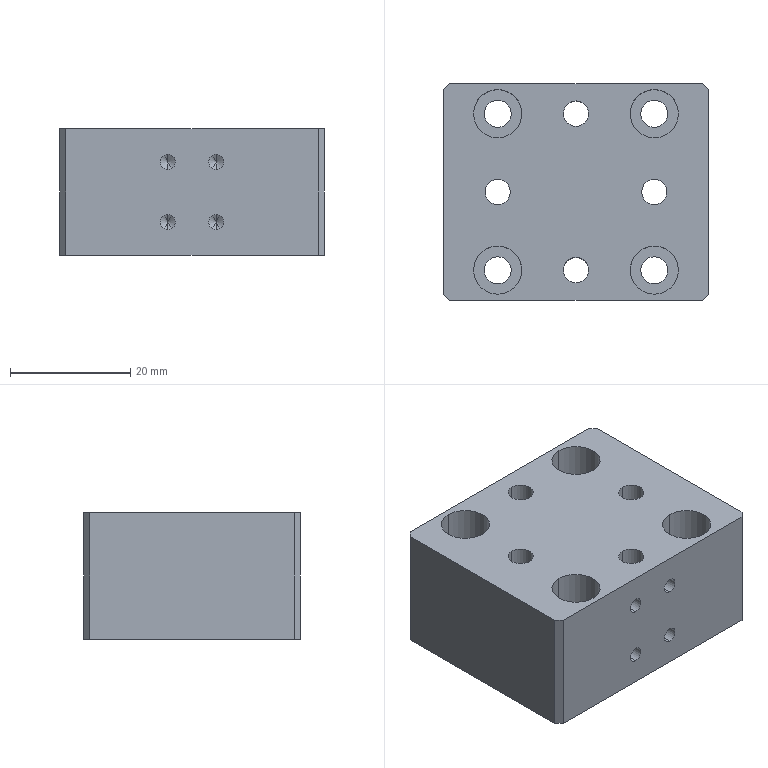Part | 1 solid | 70 faces | box 44 x 36 x 21 mm | volume 28356 mm3 | cylinder 40 | cone 16 | plane 14 | commonest cylinder face diameters 2.5 x16 4.2 x8 4.5 x8 8 x8